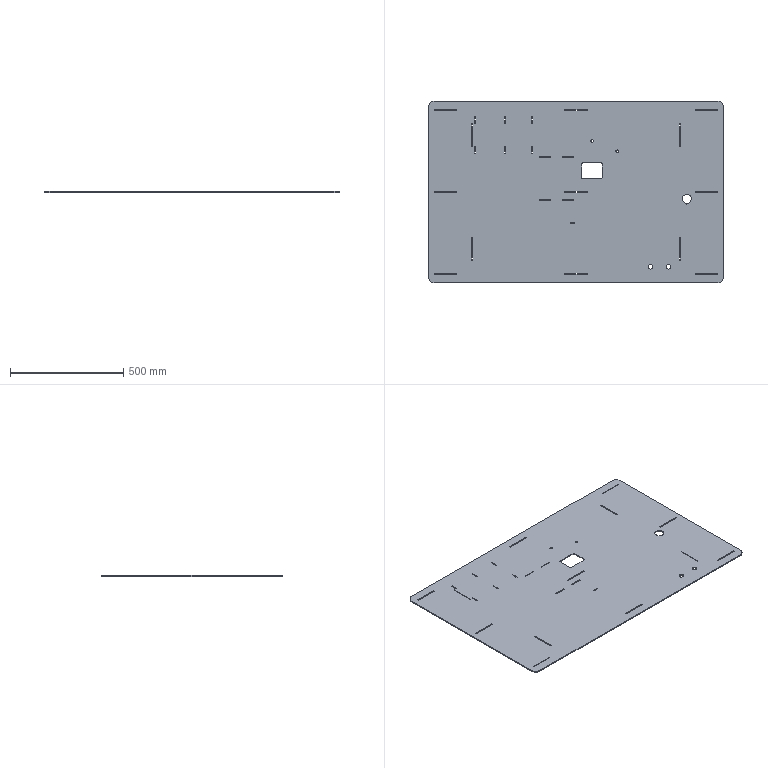Part | SolidWorks | features FlatPattern 1, SMBaseFlange 1, SheetMetal 1 | 1 solid | 127 faces | box 1300 x 800 x 4.5 mm | volume 4605383 mm3 | plane 108 | cylinder 19 | commonest cylinder face diameters 10 x4 12 x4 20 x4 50 x4 40 x3